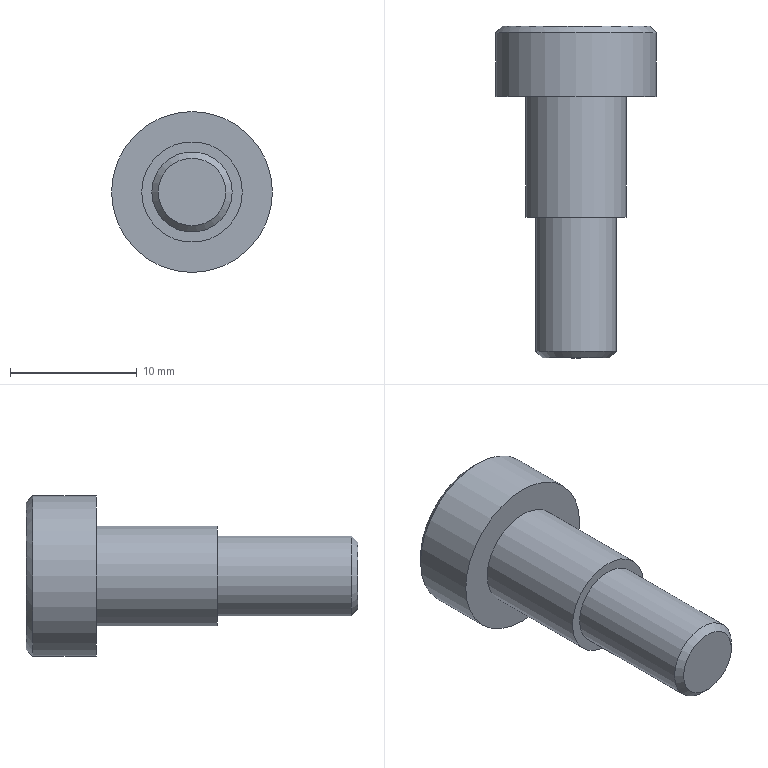Part | NX | features shoulder bolts MS51576(94035A303) 2 | 1 solid | 16 faces | box 12.7 x 26.194 x 12.7 mm | volume 1476 mm3 | plane 11 | cylinder 3 | cone 2 | commonest cylinder face diameters 6.35 x1 7.938 x1 12.7 x1
STEP:
#1=CARTESIAN_POINT('',(5.842,5.556,0.));
#2=VERTEX_POINT('',#1);
#3=CARTESIAN_POINT('',(0.,5.556,0.));
#4=DIRECTION('',(0.,-1.,0.));
#5=DIRECTION('',(1.,0.,0.));
#6=AXIS2_PLACEMENT_3D('',#3,#4,#5);
#7=CIRCLE('',#6,5.842);
#8=EDGE_CURVE('',#2,#2,#7,.F.);
#9=ORIENTED_EDGE('',*,*,#8,.T.);
#10=EDGE_LOOP('',(#9));
#11=FACE_BOUND('',#10,.T.);
#12=CARTESIAN_POINT('',(0.,5.556,-2.291));
#13=VERTEX_POINT('',#12);
#14=CARTESIAN_POINT('',(-1.984,5.556,-1.146));
#15=VERTEX_POINT('',#14);
#16=CARTESIAN_POINT('',(0.,5.556,-2.291));
#17=DIRECTION('',(-0.866,0.,0.5));
#18=VECTOR('',#17,1000.);
#19=LINE('',#16,#18);
#20=EDGE_CURVE('',#13,#15,#19,.T.);
#21=ORIENTED_EDGE('',*,*,#20,.F.);
#22=CARTESIAN_POINT('',(1.984,5.556,-1.146));
#23=VERTEX_POINT('',#22);
#24=CARTESIAN_POINT('',(1.984,5.556,-1.146));
#25=DIRECTION('',(-0.866,0.,-0.5));
#26=VECTOR('',#25,1000.);
#27=LINE('',#24,#26);
#28=EDGE_CURVE('',#23,#13,#27,.T.);
#29=ORIENTED_EDGE('',*,*,#28,.F.);
#30=CARTESIAN_POINT('',(1.984,5.556,1.146));
#31=VERTEX_POINT('',#30);
#32=CARTESIAN_POINT('',(1.984,5.556,1.146));
#33=DIRECTION('',(0.,0.,-1.));
#34=VECTOR('',#33,1000.);
#35=LINE('',#32,#34);
#36=EDGE_CURVE('',#31,#23,#35,.T.);
#37=ORIENTED_EDGE('',*,*,#36,.F.);
#38=CARTESIAN_POINT('',(0.,5.556,2.291));
#39=VERTEX_POINT('',#38);
#40=CARTESIAN_POINT('',(0.,5.556,2.291));
#41=DIRECTION('',(0.866,0.,-0.5));
#42=VECTOR('',#41,1000.);
#43=LINE('',#40,#42);
#44=EDGE_CURVE('',#39,#31,#43,.T.);
#45=ORIENTED_EDGE('',*,*,#44,.F.);
#46=CARTESIAN_POINT('',(-1.984,5.556,1.146));
#47=VERTEX_POINT('',#46);
#48=CARTESIAN_POINT('',(-1.984,5.556,1.146));
#49=DIRECTION('',(0.866,0.,0.5));
#50=VECTOR('',#49,1000.);
#51=LINE('',#48,#50);
#52=EDGE_CURVE('',#47,#39,#51,.T.);
#53=ORIENTED_EDGE('',*,*,#52,.F.);
#54=CARTESIAN_POINT('',(-1.984,5.556,-1.146));
#55=DIRECTION('',(0.,0.,1.));
#56=VECTOR('',#55,1000.);
#57=LINE('',#54,#56);
#58=EDGE_CURVE('',#15,#47,#57,.T.);
#59=ORIENTED_EDGE('',*,*,#58,.F.);
#60=EDGE_LOOP('',(#21,#29,#37,#45,#53,#59));
#61=FACE_BOUND('',#60,.T.);
#62=CARTESIAN_POINT('',(6.35,5.556,0.));
#63=DIRECTION('',(0.,-1.,0.));
#64=DIRECTION('',(1.,0.,0.));
#65=AXIS2_PLACEMENT_3D('',#62,#63,#64);
#66=PLANE('',#65);
#67=ADVANCED_FACE('',(#11,#61),#66,.F.);
#68=CARTESIAN_POINT('',(6.35,5.048,0.));
#69=VERTEX_POINT('',#68);
#70=CARTESIAN_POINT('',(0.,5.048,0.));
#71=DIRECTION('',(0.,-1.,0.));
#72=DIRECTION('',(1.,0.,0.));
#73=AXIS2_PLACEMENT_3D('',#70,#71,#72);
#74=CIRCLE('',#73,6.35);
#75=EDGE_CURVE('',#69,#69,#74,.T.);
#76=ORIENTED_EDGE('',*,*,#75,.T.);
#77=EDGE_LOOP('',(#76));
#78=FACE_BOUND('',#77,.T.);
#79=CARTESIAN_POINT('',(-6.35,0.,0.));
#80=VERTEX_POINT('',#79);
#81=CARTESIAN_POINT('',(0.,0.,0.));
#82=DIRECTION('',(0.,1.,0.));
#83=DIRECTION('',(-1.,0.,0.));
#84=AXIS2_PLACEMENT_3D('',#81,#82,#83);
#85=CIRCLE('',#84,6.35);
#86=EDGE_CURVE('',#80,#80,#85,.T.);
#87=ORIENTED_EDGE('',*,*,#86,.T.);
#88=EDGE_LOOP('',(#87));
#89=FACE_BOUND('',#88,.T.);
#90=CARTESIAN_POINT('',(0.,0.,0.));
#91=DIRECTION('',(0.,1.,0.));
#92=DIRECTION('',(-1.,0.,0.));
#93=AXIS2_PLACEMENT_3D('',#90,#91,#92);
#94=CYLINDRICAL_SURFACE('',#93,6.35);
#95=ADVANCED_FACE('',(#78,#89),#94,.T.);
#96=ORIENTED_EDGE('',*,*,#86,.F.);
#97=EDGE_LOOP('',(#96));
#98=FACE_BOUND('',#97,.T.);
#99=CARTESIAN_POINT('',(-3.969,0.,0.));
#100=VERTEX_POINT('',#99);
#101=CARTESIAN_POINT('',(0.,0.,0.));
#102=DIRECTION('',(0.,1.,0.));
#103=DIRECTION('',(-1.,0.,0.));
#104=AXIS2_PLACEMENT_3D('',#101,#102,#103);
#105=CIRCLE('',#104,3.969);
#106=EDGE_CURVE('',#100,#100,#105,.T.);
#107=ORIENTED_EDGE('',*,*,#106,.T.);
#108=EDGE_LOOP('',(#107));
#109=FACE_BOUND('',#108,.T.);
#110=CARTESIAN_POINT('',(3.969,0.,0.));
#111=DIRECTION('',(0.,1.,0.));
#112=DIRECTION('',(-1.,0.,0.));
#113=AXIS2_PLACEMENT_3D('',#110,#111,#112);
#114=PLANE('',#113);
#115=ADVANCED_FACE('',(#98,#109),#114,.F.);
#116=ORIENTED_EDGE('',*,*,#106,.F.);
#117=EDGE_LOOP('',(#116));
#118=FACE_BOUND('',#117,.T.);
#119=CARTESIAN_POINT('',(-3.969,-9.525,0.));
#120=VERTEX_POINT('',#119);
#121=CARTESIAN_POINT('',(0.,-9.525,0.));
#122=DIRECTION('',(0.,1.,0.));
#123=DIRECTION('',(-1.,0.,0.));
#124=AXIS2_PLACEMENT_3D('',#121,#122,#123);
#125=CIRCLE('',#124,3.969);
#126=EDGE_CURVE('',#120,#120,#125,.T.);
#127=ORIENTED_EDGE('',*,*,#126,.T.);
#128=EDGE_LOOP('',(#127));
#129=FACE_BOUND('',#128,.T.);
#130=CARTESIAN_POINT('',(0.,0.,0.));
#131=DIRECTION('',(0.,1.,0.));
#132=DIRECTION('',(-1.,0.,0.));
#133=AXIS2_PLACEMENT_3D('',#130,#131,#132);
#134=CYLINDRICAL_SURFACE('',#133,3.969);
#135=ADVANCED_FACE('',(#118,#129),#134,.T.);
#136=ORIENTED_EDGE('',*,*,#126,.F.);
#137=EDGE_LOOP('',(#136));
#138=FACE_BOUND('',#137,.T.);
#139=CARTESIAN_POINT('',(-3.175,-9.525,0.));
#140=VERTEX_POINT('',#139);
#141=CARTESIAN_POINT('',(0.,-9.525,0.));
#142=DIRECTION('',(0.,1.,0.));
#143=DIRECTION('',(-1.,0.,0.));
#144=AXIS2_PLACEMENT_3D('',#141,#142,#143);
#145=CIRCLE('',#144,3.175);
#146=EDGE_CURVE('',#140,#140,#145,.T.);
#147=ORIENTED_EDGE('',*,*,#146,.T.);
#148=EDGE_LOOP('',(#147));
#149=FACE_BOUND('',#148,.T.);
#150=CARTESIAN_POINT('',(3.175,-9.525,0.));
#151=DIRECTION('',(0.,1.,0.));
#152=DIRECTION('',(-1.,0.,0.));
#153=AXIS2_PLACEMENT_3D('',#150,#151,#152);
#154=PLANE('',#153);
#155=ADVANCED_FACE('',(#138,#149),#154,.F.);
#156=CARTESIAN_POINT('',(-3.175,-20.13,0.));
#157=VERTEX_POINT('',#156);
#158=CARTESIAN_POINT('',(0.,-20.13,0.));
#159=DIRECTION('',(0.,1.,0.));
#160=DIRECTION('',(-1.,0.,0.));
#161=AXIS2_PLACEMENT_3D('',#158,#159,#160);
#162=CIRCLE('',#161,3.175);
#163=EDGE_CURVE('',#157,#157,#162,.T.);
#164=ORIENTED_EDGE('',*,*,#163,.T.);
#165=EDGE_LOOP('',(#164));
#166=FACE_BOUND('',#165,.T.);
#167=ORIENTED_EDGE('',*,*,#146,.F.);
#168=EDGE_LOOP('',(#167));
#169=FACE_BOUND('',#168,.T.);
#170=CARTESIAN_POINT('',(0.,0.,0.));
#171=DIRECTION('',(0.,1.,0.));
#172=DIRECTION('',(-1.,0.,0.));
#173=AXIS2_PLACEMENT_3D('',#170,#171,#172);
#174=CYLINDRICAL_SURFACE('',#173,3.175);
#175=ADVANCED_FACE('',(#166,#169),#174,.T.);
#176=CARTESIAN_POINT('',(-2.667,-20.637,0.));
#177=VERTEX_POINT('',#176);
#178=CARTESIAN_POINT('',(0.,-20.637,0.));
#179=DIRECTION('',(0.,1.,0.));
#180=DIRECTION('',(-1.,0.,0.));
#181=AXIS2_PLACEMENT_3D('',#178,#179,#180);
#182=CIRCLE('',#181,2.667);
#183=EDGE_CURVE('',#177,#177,#182,.F.);
#184=ORIENTED_EDGE('',*,*,#183,.T.);
#185=EDGE_LOOP('',(#184));
#186=FACE_BOUND('',#185,.T.);
#187=CARTESIAN_POINT('',(0.,-20.637,0.));
#188=DIRECTION('',(0.,1.,0.));
#189=DIRECTION('',(-1.,0.,0.));
#190=AXIS2_PLACEMENT_3D('',#187,#188,#189);
#191=PLANE('',#190);
#192=ADVANCED_FACE('',(#186),#191,.F.);
#193=ORIENTED_EDGE('',*,*,#28,.T.);
#194=CARTESIAN_POINT('',(0.,2.381,-2.291));
#195=VERTEX_POINT('',#194);
#196=CARTESIAN_POINT('',(0.,2.381,-2.291));
#197=DIRECTION('',(0.,1.,0.));
#198=VECTOR('',#197,1000.);
#199=LINE('',#196,#198);
#200=EDGE_CURVE('',#195,#13,#199,.T.);
#201=ORIENTED_EDGE('',*,*,#200,.F.);
#202=CARTESIAN_POINT('',(1.984,2.381,-1.146));
#203=VERTEX_POINT('',#202);
#204=CARTESIAN_POINT('',(1.984,2.381,-1.146));
#205=DIRECTION('',(-0.866,0.,-0.5));
#206=VECTOR('',#205,1000.);
#207=LINE('',#204,#206);
#208=EDGE_CURVE('',#203,#195,#207,.T.);
#209=ORIENTED_EDGE('',*,*,#208,.F.);
#210=CARTESIAN_POINT('',(1.984,2.381,-1.146));
#211=DIRECTION('',(0.,1.,0.));
#212=VECTOR('',#211,1000.);
#213=LINE('',#210,#212);
#214=EDGE_CURVE('',#203,#23,#213,.T.);
#215=ORIENTED_EDGE('',*,*,#214,.T.);
#216=EDGE_LOOP('',(#193,#201,#209,#215));
#217=FACE_BOUND('',#216,.T.);
#218=CARTESIAN_POINT('',(1.984,2.381,-1.146));
#219=DIRECTION('',(0.5,0.,-0.866));
#220=DIRECTION('',(-0.866,0.,-0.5));
#221=AXIS2_PLACEMENT_3D('',#218,#219,#220);
#222=PLANE('',#221);
#223=ADVANCED_FACE('',(#217),#222,.F.);
#224=ORIENTED_EDGE('',*,*,#36,.T.);
#225=ORIENTED_EDGE('',*,*,#214,.F.);
#226=CARTESIAN_POINT('',(1.984,2.381,1.146));
#227=VERTEX_POINT('',#226);
#228=CARTESIAN_POINT('',(1.984,2.381,1.146));
#229=DIRECTION('',(0.,0.,-1.));
#230=VECTOR('',#229,1000.);
#231=LINE('',#228,#230);
#232=EDGE_CURVE('',#227,#203,#231,.T.);
#233=ORIENTED_EDGE('',*,*,#232,.F.);
#234=CARTESIAN_POINT('',(1.984,2.381,1.146));
#235=DIRECTION('',(0.,1.,0.));
#236=VECTOR('',#235,1000.);
#237=LINE('',#234,#236);
#238=EDGE_CURVE('',#227,#31,#237,.T.);
#239=ORIENTED_EDGE('',*,*,#238,.T.);
#240=EDGE_LOOP('',(#224,#225,#233,#239));
#241=FACE_BOUND('',#240,.T.);
#242=CARTESIAN_POINT('',(1.984,2.381,1.146));
#243=DIRECTION('',(1.,0.,0.));
#244=DIRECTION('',(0.,1.,0.));
#245=AXIS2_PLACEMENT_3D('',#242,#243,#244);
#246=PLANE('',#245);
#247=ADVANCED_FACE('',(#241),#246,.F.);
#248=ORIENTED_EDGE('',*,*,#44,.T.);
#249=ORIENTED_EDGE('',*,*,#238,.F.);
#250=CARTESIAN_POINT('',(0.,2.381,2.291));
#251=VERTEX_POINT('',#250);
#252=CARTESIAN_POINT('',(0.,2.381,2.291));
#253=DIRECTION('',(0.866,0.,-0.5));
#254=VECTOR('',#253,1000.);
#255=LINE('',#252,#254);
#256=EDGE_CURVE('',#251,#227,#255,.T.);
#257=ORIENTED_EDGE('',*,*,#256,.F.);
#258=CARTESIAN_POINT('',(0.,2.381,2.291));
#259=DIRECTION('',(0.,1.,0.));
#260=VECTOR('',#259,1000.);
#261=LINE('',#258,#260);
#262=EDGE_CURVE('',#251,#39,#261,.T.);
#263=ORIENTED_EDGE('',*,*,#262,.T.);
#264=EDGE_LOOP('',(#248,#249,#257,#263));
#265=FACE_BOUND('',#264,.T.);
#266=CARTESIAN_POINT('',(0.,2.381,2.291));
#267=DIRECTION('',(0.5,0.,0.866));
#268=DIRECTION('',(0.866,0.,-0.5));
#269=AXIS2_PLACEMENT_3D('',#266,#267,#268);
#270=PLANE('',#269);
#271=ADVANCED_FACE('',(#265),#270,.F.);
#272=ORIENTED_EDGE('',*,*,#52,.T.);
#273=ORIENTED_EDGE('',*,*,#262,.F.);
#274=CARTESIAN_POINT('',(-1.984,2.381,1.146));
#275=VERTEX_POINT('',#274);
#276=CARTESIAN_POINT('',(-1.984,2.381,1.146));
#277=DIRECTION('',(0.866,0.,0.5));
#278=VECTOR('',#277,1000.);
#279=LINE('',#276,#278);
#280=EDGE_CURVE('',#275,#251,#279,.T.);
#281=ORIENTED_EDGE('',*,*,#280,.F.);
#282=CARTESIAN_POINT('',(-1.984,2.381,1.146));
#283=DIRECTION('',(0.,1.,0.));
#284=VECTOR('',#283,1000.);
#285=LINE('',#282,#284);
#286=EDGE_CURVE('',#275,#47,#285,.T.);
#287=ORIENTED_EDGE('',*,*,#286,.T.);
#288=EDGE_LOOP('',(#272,#273,#281,#287));
#289=FACE_BOUND('',#288,.T.);
#290=CARTESIAN_POINT('',(-1.984,2.381,1.146));
#291=DIRECTION('',(-0.5,0.,0.866));
#292=DIRECTION('',(0.866,0.,0.5));
#293=AXIS2_PLACEMENT_3D('',#290,#291,#292);
#294=PLANE('',#293);
#295=ADVANCED_FACE('',(#289),#294,.F.);
#296=ORIENTED_EDGE('',*,*,#58,.T.);
#297=ORIENTED_EDGE('',*,*,#286,.F.);
#298=CARTESIAN_POINT('',(-1.984,2.381,-1.146));
#299=VERTEX_POINT('',#298);
#300=CARTESIAN_POINT('',(-1.984,2.381,-1.146));
#301=DIRECTION('',(0.,0.,1.));
#302=VECTOR('',#301,1000.);
#303=LINE('',#300,#302);
#304=EDGE_CURVE('',#299,#275,#303,.T.);
#305=ORIENTED_EDGE('',*,*,#304,.F.);
#306=CARTESIAN_POINT('',(-1.984,2.381,-1.146));
#307=DIRECTION('',(0.,1.,0.));
#308=VECTOR('',#307,1000.);
#309=LINE('',#306,#308);
#310=EDGE_CURVE('',#299,#15,#309,.T.);
#311=ORIENTED_EDGE('',*,*,#310,.T.);
#312=EDGE_LOOP('',(#296,#297,#305,#311));
#313=FACE_BOUND('',#312,.T.);
#314=CARTESIAN_POINT('',(-1.984,2.381,-1.146));
#315=DIRECTION('',(-1.,0.,0.));
#316=DIRECTION('',(0.,-1.,0.));
#317=AXIS2_PLACEMENT_3D('',#314,#315,#316);
#318=PLANE('',#317);
#319=ADVANCED_FACE('',(#313),#318,.F.);
#320=ORIENTED_EDGE('',*,*,#20,.T.);
#321=ORIENTED_EDGE('',*,*,#310,.F.);
#322=CARTESIAN_POINT('',(0.,2.381,-2.291));
#323=DIRECTION('',(-0.866,0.,0.5));
#324=VECTOR('',#323,1000.);
#325=LINE('',#322,#324);
#326=EDGE_CURVE('',#195,#299,#325,.T.);
#327=ORIENTED_EDGE('',*,*,#326,.F.);
#328=ORIENTED_EDGE('',*,*,#200,.T.);
#329=EDGE_LOOP('',(#320,#321,#327,#328));
#330=FACE_BOUND('',#329,.T.);
#331=CARTESIAN_POINT('',(0.,2.381,-2.291));
#332=DIRECTION('',(-0.5,0.,-0.866));
#333=DIRECTION('',(-0.866,0.,0.5));
#334=AXIS2_PLACEMENT_3D('',#331,#332,#333);
#335=PLANE('',#334);
#336=ADVANCED_FACE('',(#330),#335,.F.);
#337=ORIENTED_EDGE('',*,*,#208,.T.);
#338=ORIENTED_EDGE('',*,*,#326,.T.);
#339=ORIENTED_EDGE('',*,*,#304,.T.);
#340=ORIENTED_EDGE('',*,*,#280,.T.);
#341=ORIENTED_EDGE('',*,*,#256,.T.);
#342=ORIENTED_EDGE('',*,*,#232,.T.);
#343=EDGE_LOOP('',(#337,#338,#339,#340,#341,#342));
#344=FACE_BOUND('',#343,.T.);
#345=CARTESIAN_POINT('',(-1.984,2.381,-3.437));
#346=DIRECTION('',(0.,1.,0.));
#347=DIRECTION('',(0.,0.,1.));
#348=AXIS2_PLACEMENT_3D('',#345,#346,#347);
#349=PLANE('',#348);
#350=ADVANCED_FACE('',(#344),#349,.T.);
#351=ORIENTED_EDGE('',*,*,#75,.F.);
#352=EDGE_LOOP('',(#351));
#353=FACE_BOUND('',#352,.T.);
#354=ORIENTED_EDGE('',*,*,#8,.F.);
#355=EDGE_LOOP('',(#354));
#356=FACE_BOUND('',#355,.T.);
#357=CARTESIAN_POINT('',(0.,5.556,0.));
#358=DIRECTION('',(0.,-1.,0.));
#359=DIRECTION('',(1.,0.,0.));
#360=AXIS2_PLACEMENT_3D('',#357,#358,#359);
#361=CONICAL_SURFACE('',#360,5.842,0.7854);
#362=ADVANCED_FACE('',(#353,#356),#361,.T.);
#363=ORIENTED_EDGE('',*,*,#183,.F.);
#364=EDGE_LOOP('',(#363));
#365=FACE_BOUND('',#364,.T.);
#366=ORIENTED_EDGE('',*,*,#163,.F.);
#367=EDGE_LOOP('',(#366));
#368=FACE_BOUND('',#367,.T.);
#369=CARTESIAN_POINT('',(0.,-20.13,0.));
#370=DIRECTION('',(0.,1.,0.));
#371=DIRECTION('',(-1.,0.,0.));
#372=AXIS2_PLACEMENT_3D('',#369,#370,#371);
#373=CONICAL_SURFACE('',#372,3.175,0.7854);
#374=ADVANCED_FACE('',(#365,#368),#373,.T.);
#375=CLOSED_SHELL('',(#67,#95,#115,#135,#155,#175,#192,#223,#247,#271,#295,#319,#336,#350,#362,#374));
#376=MANIFOLD_SOLID_BREP('',#375);
#377=(LENGTH_UNIT()NAMED_UNIT(*)SI_UNIT(.MILLI.,.METRE.));
#378=UNCERTAINTY_MEASURE_WITH_UNIT(LENGTH_MEASURE(0.00001),#377,'','');
#379=(NAMED_UNIT(*)PLANE_ANGLE_UNIT()SI_UNIT($,.RADIAN.));
#380=(NAMED_UNIT(*)SI_UNIT($,.STERADIAN.)SOLID_ANGLE_UNIT());
#381=(GEOMETRIC_REPRESENTATION_CONTEXT(3)GLOBAL_UNCERTAINTY_ASSIGNED_CONTEXT((#378))GLOBAL_UNIT_ASSIGNED_CONTEXT((#377,#379,#380))REPRESENTATION_CONTEXT('',''));
#382=ADVANCED_BREP_SHAPE_REPRESENTATION('',(#376),#381);